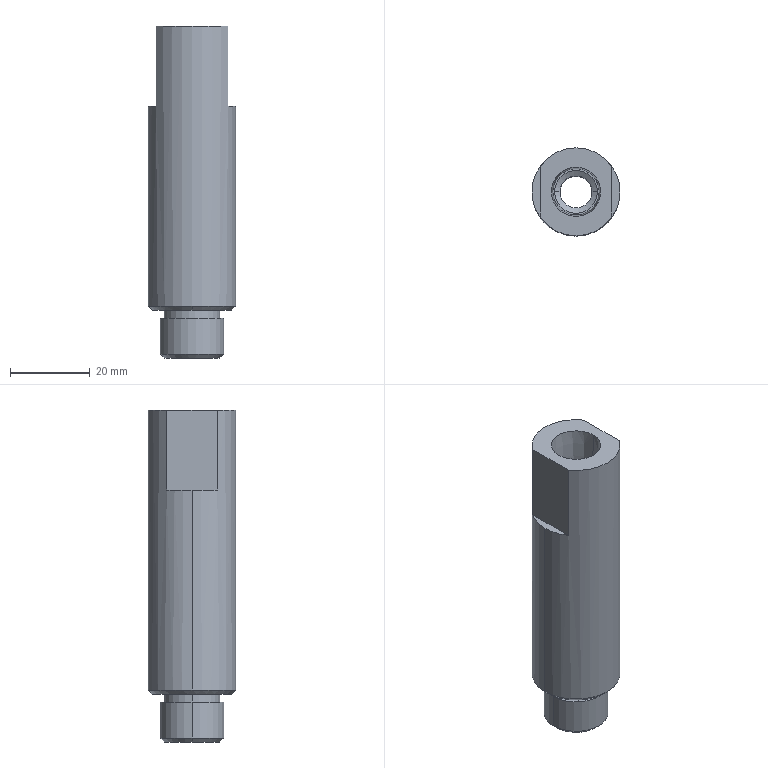Part | SolidWorks | features BaseBody 1 | 1 solid | 27 faces | box 22 x 22 x 83 mm | volume 23413 mm3 | cylinder 10 | plane 9 | cone 8 | commonest cylinder face diameters 8 x2 10.7 x2 14 x2 16 x2 22 x2
STEP:
#1=CARTESIAN_POINT('',(9.,6.325,63.));
#2=VERTEX_POINT('',#1);
#3=CARTESIAN_POINT('',(11.,0.,63.));
#4=VERTEX_POINT('',#3);
#5=CARTESIAN_POINT('',(0.,0.,63.));
#6=DIRECTION('',(0.,0.,-1.));
#7=DIRECTION('',(-1.,0.,0.));
#8=AXIS2_PLACEMENT_3D('',#5,#6,#7);
#9=CIRCLE('',#8,11.);
#10=EDGE_CURVE('',#2,#4,#9,.T.);
#11=ORIENTED_EDGE('',*,*,#10,.T.);
#12=CARTESIAN_POINT('',(11.,0.,13.));
#13=VERTEX_POINT('',#12);
#14=CARTESIAN_POINT('',(11.,0.,83.));
#15=DIRECTION('',(0.,0.,-1.));
#16=VECTOR('',#15,1000.);
#17=LINE('',#14,#16);
#18=EDGE_CURVE('',#4,#13,#17,.T.);
#19=ORIENTED_EDGE('',*,*,#18,.T.);
#20=CARTESIAN_POINT('',(0.,11.,13.));
#21=VERTEX_POINT('',#20);
#22=CARTESIAN_POINT('',(0.,0.,13.));
#23=DIRECTION('',(0.,0.,1.));
#24=DIRECTION('',(-1.,0.,0.));
#25=AXIS2_PLACEMENT_3D('',#22,#23,#24);
#26=CIRCLE('',#25,11.);
#27=EDGE_CURVE('',#13,#21,#26,.T.);
#28=ORIENTED_EDGE('',*,*,#27,.T.);
#29=CARTESIAN_POINT('',(-11.,0.,13.));
#30=VERTEX_POINT('',#29);
#31=CARTESIAN_POINT('',(0.,0.,13.));
#32=DIRECTION('',(0.,0.,1.));
#33=DIRECTION('',(-1.,0.,0.));
#34=AXIS2_PLACEMENT_3D('',#31,#32,#33);
#35=CIRCLE('',#34,11.);
#36=EDGE_CURVE('',#21,#30,#35,.T.);
#37=ORIENTED_EDGE('',*,*,#36,.T.);
#38=CARTESIAN_POINT('',(-11.,0.,63.));
#39=VERTEX_POINT('',#38);
#40=CARTESIAN_POINT('',(-11.,0.,83.));
#41=DIRECTION('',(0.,0.,-1.));
#42=VECTOR('',#41,1000.);
#43=LINE('',#40,#42);
#44=EDGE_CURVE('',#39,#30,#43,.T.);
#45=ORIENTED_EDGE('',*,*,#44,.F.);
#46=CARTESIAN_POINT('',(-9.,6.325,63.));
#47=VERTEX_POINT('',#46);
#48=CARTESIAN_POINT('',(0.,0.,63.));
#49=DIRECTION('',(0.,0.,-1.));
#50=DIRECTION('',(-1.,0.,0.));
#51=AXIS2_PLACEMENT_3D('',#48,#49,#50);
#52=CIRCLE('',#51,11.);
#53=EDGE_CURVE('',#39,#47,#52,.T.);
#54=ORIENTED_EDGE('',*,*,#53,.T.);
#55=CARTESIAN_POINT('',(-9.,6.325,83.));
#56=VERTEX_POINT('',#55);
#57=CARTESIAN_POINT('',(-9.,6.325,83.));
#58=DIRECTION('',(0.,0.,1.));
#59=VECTOR('',#58,1000.);
#60=LINE('',#57,#59);
#61=EDGE_CURVE('',#47,#56,#60,.T.);
#62=ORIENTED_EDGE('',*,*,#61,.T.);
#63=CARTESIAN_POINT('',(9.,6.325,83.));
#64=VERTEX_POINT('',#63);
#65=CARTESIAN_POINT('',(0.,0.,83.));
#66=DIRECTION('',(0.,0.,-1.));
#67=DIRECTION('',(-1.,0.,0.));
#68=AXIS2_PLACEMENT_3D('',#65,#66,#67);
#69=CIRCLE('',#68,11.);
#70=EDGE_CURVE('',#56,#64,#69,.T.);
#71=ORIENTED_EDGE('',*,*,#70,.T.);
#72=CARTESIAN_POINT('',(9.,6.325,83.));
#73=DIRECTION('',(0.,0.,-1.));
#74=VECTOR('',#73,1000.);
#75=LINE('',#72,#74);
#76=EDGE_CURVE('',#64,#2,#75,.T.);
#77=ORIENTED_EDGE('',*,*,#76,.T.);
#78=EDGE_LOOP('',(#11,#19,#28,#37,#45,#54,#62,#71,#77));
#79=FACE_OUTER_BOUND('',#78,.T.);
#80=CARTESIAN_POINT('',(0.,0.,83.));
#81=DIRECTION('',(0.,0.,-1.));
#82=DIRECTION('',(-1.,0.,0.));
#83=AXIS2_PLACEMENT_3D('',#80,#81,#82);
#84=CYLINDRICAL_SURFACE('',#83,11.);
#85=ADVANCED_FACE('',(#79),#84,.T.);
#86=CARTESIAN_POINT('',(0.,-10.,12.));
#87=VERTEX_POINT('',#86);
#88=CARTESIAN_POINT('',(0.,10.,12.));
#89=VERTEX_POINT('',#88);
#90=CARTESIAN_POINT('',(0.,0.,12.));
#91=DIRECTION('',(0.,0.,1.));
#92=DIRECTION('',(0.,-1.,0.));
#93=AXIS2_PLACEMENT_3D('',#90,#91,#92);
#94=CIRCLE('',#93,10.);
#95=EDGE_CURVE('',#87,#89,#94,.T.);
#96=ORIENTED_EDGE('',*,*,#95,.T.);
#97=CARTESIAN_POINT('',(0.,11.,13.));
#98=DIRECTION('',(0.,0.7071,0.7071));
#99=VECTOR('',#98,1000.);
#100=LINE('',#97,#99);
#101=EDGE_CURVE('',#89,#21,#100,.T.);
#102=ORIENTED_EDGE('',*,*,#101,.T.);
#103=ORIENTED_EDGE('',*,*,#27,.F.);
#104=CARTESIAN_POINT('',(0.,-11.,13.));
#105=VERTEX_POINT('',#104);
#106=CARTESIAN_POINT('',(0.,0.,13.));
#107=DIRECTION('',(0.,0.,1.));
#108=DIRECTION('',(-1.,0.,0.));
#109=AXIS2_PLACEMENT_3D('',#106,#107,#108);
#110=CIRCLE('',#109,11.);
#111=EDGE_CURVE('',#105,#13,#110,.T.);
#112=ORIENTED_EDGE('',*,*,#111,.F.);
#113=CARTESIAN_POINT('',(0.,-11.,13.));
#114=DIRECTION('',(0.,-0.7071,0.7071));
#115=VECTOR('',#114,1000.);
#116=LINE('',#113,#115);
#117=EDGE_CURVE('',#87,#105,#116,.T.);
#118=ORIENTED_EDGE('',*,*,#117,.F.);
#119=EDGE_LOOP('',(#96,#102,#103,#112,#118));
#120=FACE_OUTER_BOUND('',#119,.T.);
#121=CARTESIAN_POINT('',(0.,0.,13.));
#122=DIRECTION('',(0.,0.,1.));
#123=DIRECTION('',(0.,-1.,0.));
#124=AXIS2_PLACEMENT_3D('',#121,#122,#123);
#125=CONICAL_SURFACE('',#124,11.,0.7854);
#126=ADVANCED_FACE('',(#120),#125,.T.);
#127=CARTESIAN_POINT('',(-5.811,0.,72.));
#128=VERTEX_POINT('',#127);
#129=CARTESIAN_POINT('',(5.811,0.,72.));
#130=VERTEX_POINT('',#129);
#131=CARTESIAN_POINT('',(0.,0.,72.));
#132=DIRECTION('',(0.,0.,1.));
#133=DIRECTION('',(1.,0.,0.));
#134=AXIS2_PLACEMENT_3D('',#131,#132,#133);
#135=CIRCLE('',#134,5.811);
#136=EDGE_CURVE('',#128,#130,#135,.T.);
#137=ORIENTED_EDGE('',*,*,#136,.F.);
#138=CARTESIAN_POINT('',(-6.154,0.,83.));
#139=VERTEX_POINT('',#138);
#140=CARTESIAN_POINT('',(-6.154,0.,83.));
#141=DIRECTION('',(-0.0312,0.,0.9995));
#142=VECTOR('',#141,1000.);
#143=LINE('',#140,#142);
#144=EDGE_CURVE('',#128,#139,#143,.T.);
#145=ORIENTED_EDGE('',*,*,#144,.T.);
#146=CARTESIAN_POINT('',(6.154,0.,83.));
#147=VERTEX_POINT('',#146);
#148=CARTESIAN_POINT('',(0.,0.,83.));
#149=DIRECTION('',(0.,0.,-1.));
#150=DIRECTION('',(1.,0.,0.));
#151=AXIS2_PLACEMENT_3D('',#148,#149,#150);
#152=CIRCLE('',#151,6.154);
#153=EDGE_CURVE('',#147,#139,#152,.T.);
#154=ORIENTED_EDGE('',*,*,#153,.F.);
#155=CARTESIAN_POINT('',(6.154,0.,83.));
#156=DIRECTION('',(0.0312,0.,0.9995));
#157=VECTOR('',#156,1000.);
#158=LINE('',#155,#157);
#159=EDGE_CURVE('',#130,#147,#158,.T.);
#160=ORIENTED_EDGE('',*,*,#159,.F.);
#161=EDGE_LOOP('',(#137,#145,#154,#160));
#162=FACE_OUTER_BOUND('',#161,.T.);
#163=CARTESIAN_POINT('',(0.,0.,83.));
#164=DIRECTION('',(0.,0.,1.));
#165=DIRECTION('',(1.,0.,0.));
#166=AXIS2_PLACEMENT_3D('',#163,#164,#165);
#167=CONICAL_SURFACE('',#166,6.154,0.03121);
#168=ADVANCED_FACE('',(#162),#167,.F.);
#169=CARTESIAN_POINT('',(-7.,0.,12.));
#170=VERTEX_POINT('',#169);
#171=CARTESIAN_POINT('',(7.,0.,12.));
#172=VERTEX_POINT('',#171);
#173=CARTESIAN_POINT('',(0.,0.,12.));
#174=DIRECTION('',(0.,0.,-1.));
#175=DIRECTION('',(-1.,0.,0.));
#176=AXIS2_PLACEMENT_3D('',#173,#174,#175);
#177=CIRCLE('',#176,7.);
#178=EDGE_CURVE('',#170,#172,#177,.T.);
#179=ORIENTED_EDGE('',*,*,#178,.T.);
#180=CARTESIAN_POINT('',(7.,0.,10.));
#181=VERTEX_POINT('',#180);
#182=CARTESIAN_POINT('',(7.,0.,0.));
#183=DIRECTION('',(0.,0.,-1.));
#184=VECTOR('',#183,1000.);
#185=LINE('',#182,#184);
#186=EDGE_CURVE('',#172,#181,#185,.T.);
#187=ORIENTED_EDGE('',*,*,#186,.T.);
#188=CARTESIAN_POINT('',(-7.,0.,10.));
#189=VERTEX_POINT('',#188);
#190=CARTESIAN_POINT('',(0.,0.,10.));
#191=DIRECTION('',(0.,0.,1.));
#192=DIRECTION('',(-1.,0.,0.));
#193=AXIS2_PLACEMENT_3D('',#190,#191,#192);
#194=CIRCLE('',#193,7.);
#195=EDGE_CURVE('',#181,#189,#194,.T.);
#196=ORIENTED_EDGE('',*,*,#195,.T.);
#197=CARTESIAN_POINT('',(-7.,0.,0.));
#198=DIRECTION('',(0.,0.,-1.));
#199=VECTOR('',#198,1000.);
#200=LINE('',#197,#199);
#201=EDGE_CURVE('',#170,#189,#200,.T.);
#202=ORIENTED_EDGE('',*,*,#201,.F.);
#203=EDGE_LOOP('',(#179,#187,#196,#202));
#204=FACE_OUTER_BOUND('',#203,.T.);
#205=CARTESIAN_POINT('',(0.,0.,0.));
#206=DIRECTION('',(0.,0.,-1.));
#207=DIRECTION('',(-1.,0.,0.));
#208=AXIS2_PLACEMENT_3D('',#205,#206,#207);
#209=CYLINDRICAL_SURFACE('',#208,7.);
#210=ADVANCED_FACE('',(#204),#209,.T.);
#211=CARTESIAN_POINT('',(-5.35,0.,65.));
#212=VERTEX_POINT('',#211);
#213=CARTESIAN_POINT('',(5.35,0.,65.));
#214=VERTEX_POINT('',#213);
#215=CARTESIAN_POINT('',(0.,0.,65.));
#216=DIRECTION('',(0.,0.,1.));
#217=DIRECTION('',(1.,0.,0.));
#218=AXIS2_PLACEMENT_3D('',#215,#216,#217);
#219=CIRCLE('',#218,5.35);
#220=EDGE_CURVE('',#212,#214,#219,.T.);
#221=ORIENTED_EDGE('',*,*,#220,.F.);
#222=CARTESIAN_POINT('',(-5.35,0.,72.));
#223=VERTEX_POINT('',#222);
#224=CARTESIAN_POINT('',(-5.35,0.,83.));
#225=DIRECTION('',(0.,0.,1.));
#226=VECTOR('',#225,1000.);
#227=LINE('',#224,#226);
#228=EDGE_CURVE('',#212,#223,#227,.T.);
#229=ORIENTED_EDGE('',*,*,#228,.T.);
#230=CARTESIAN_POINT('',(5.35,0.,72.));
#231=VERTEX_POINT('',#230);
#232=CARTESIAN_POINT('',(0.,0.,72.));
#233=DIRECTION('',(0.,0.,1.));
#234=DIRECTION('',(1.,0.,0.));
#235=AXIS2_PLACEMENT_3D('',#232,#233,#234);
#236=CIRCLE('',#235,5.35);
#237=EDGE_CURVE('',#223,#231,#236,.T.);
#238=ORIENTED_EDGE('',*,*,#237,.T.);
#239=CARTESIAN_POINT('',(5.35,0.,83.));
#240=DIRECTION('',(0.,0.,1.));
#241=VECTOR('',#240,1000.);
#242=LINE('',#239,#241);
#243=EDGE_CURVE('',#214,#231,#242,.T.);
#244=ORIENTED_EDGE('',*,*,#243,.F.);
#245=EDGE_LOOP('',(#221,#229,#238,#244));
#246=FACE_OUTER_BOUND('',#245,.T.);
#247=CARTESIAN_POINT('',(0.,0.,83.));
#248=DIRECTION('',(0.,0.,1.));
#249=DIRECTION('',(1.,0.,0.));
#250=AXIS2_PLACEMENT_3D('',#247,#248,#249);
#251=CYLINDRICAL_SURFACE('',#250,5.35);
#252=ADVANCED_FACE('',(#246),#251,.F.);
#253=CARTESIAN_POINT('',(-4.,0.,64.189));
#254=VERTEX_POINT('',#253);
#255=CARTESIAN_POINT('',(4.,0.,64.189));
#256=VERTEX_POINT('',#255);
#257=CARTESIAN_POINT('',(0.,0.,64.189));
#258=DIRECTION('',(0.,0.,1.));
#259=DIRECTION('',(1.,0.,0.));
#260=AXIS2_PLACEMENT_3D('',#257,#258,#259);
#261=CIRCLE('',#260,4.);
#262=EDGE_CURVE('',#254,#256,#261,.T.);
#263=ORIENTED_EDGE('',*,*,#262,.F.);
#264=CARTESIAN_POINT('',(-5.35,0.,65.));
#265=DIRECTION('',(-0.8572,0.,0.515));
#266=VECTOR('',#265,1000.);
#267=LINE('',#264,#266);
#268=EDGE_CURVE('',#254,#212,#267,.T.);
#269=ORIENTED_EDGE('',*,*,#268,.T.);
#270=ORIENTED_EDGE('',*,*,#220,.T.);
#271=CARTESIAN_POINT('',(5.35,0.,65.));
#272=DIRECTION('',(0.8572,0.,0.515));
#273=VECTOR('',#272,1000.);
#274=LINE('',#271,#273);
#275=EDGE_CURVE('',#256,#214,#274,.T.);
#276=ORIENTED_EDGE('',*,*,#275,.F.);
#277=EDGE_LOOP('',(#263,#269,#270,#276));
#278=FACE_OUTER_BOUND('',#277,.T.);
#279=CARTESIAN_POINT('',(0.,0.,65.));
#280=DIRECTION('',(0.,0.,1.));
#281=DIRECTION('',(1.,0.,0.));
#282=AXIS2_PLACEMENT_3D('',#279,#280,#281);
#283=CONICAL_SURFACE('',#282,5.35,1.03);
#284=ADVANCED_FACE('',(#278),#283,.F.);
#285=CARTESIAN_POINT('',(8.,0.,10.));
#286=VERTEX_POINT('',#285);
#287=CARTESIAN_POINT('',(-8.,0.,10.));
#288=VERTEX_POINT('',#287);
#289=CARTESIAN_POINT('',(0.,0.,10.));
#290=DIRECTION('',(0.,0.,1.));
#291=DIRECTION('',(-1.,0.,0.));
#292=AXIS2_PLACEMENT_3D('',#289,#290,#291);
#293=CIRCLE('',#292,8.);
#294=EDGE_CURVE('',#286,#288,#293,.T.);
#295=ORIENTED_EDGE('',*,*,#294,.F.);
#296=CARTESIAN_POINT('',(8.,0.,1.));
#297=VERTEX_POINT('',#296);
#298=CARTESIAN_POINT('',(8.,0.,12.));
#299=DIRECTION('',(0.,0.,-1.));
#300=VECTOR('',#299,1000.);
#301=LINE('',#298,#300);
#302=EDGE_CURVE('',#286,#297,#301,.T.);
#303=ORIENTED_EDGE('',*,*,#302,.T.);
#304=CARTESIAN_POINT('',(-8.,0.,1.));
#305=VERTEX_POINT('',#304);
#306=CARTESIAN_POINT('',(0.,0.,1.));
#307=DIRECTION('',(0.,0.,1.));
#308=DIRECTION('',(-1.,0.,0.));
#309=AXIS2_PLACEMENT_3D('',#306,#307,#308);
#310=CIRCLE('',#309,8.);
#311=EDGE_CURVE('',#297,#305,#310,.T.);
#312=ORIENTED_EDGE('',*,*,#311,.T.);
#313=CARTESIAN_POINT('',(-8.,0.,12.));
#314=DIRECTION('',(0.,0.,-1.));
#315=VECTOR('',#314,1000.);
#316=LINE('',#313,#315);
#317=EDGE_CURVE('',#288,#305,#316,.T.);
#318=ORIENTED_EDGE('',*,*,#317,.F.);
#319=EDGE_LOOP('',(#295,#303,#312,#318));
#320=FACE_OUTER_BOUND('',#319,.T.);
#321=CARTESIAN_POINT('',(0.,0.,12.));
#322=DIRECTION('',(0.,0.,-1.));
#323=DIRECTION('',(-1.,0.,0.));
#324=AXIS2_PLACEMENT_3D('',#321,#322,#323);
#325=CYLINDRICAL_SURFACE('',#324,8.);
#326=ADVANCED_FACE('',(#320),#325,.T.);
#327=ORIENTED_EDGE('',*,*,#262,.T.);
#328=CARTESIAN_POINT('',(4.,0.,0.));
#329=VERTEX_POINT('',#328);
#330=CARTESIAN_POINT('',(4.,0.,0.));
#331=DIRECTION('',(0.,0.,-1.));
#332=VECTOR('',#331,1000.);
#333=LINE('',#330,#332);
#334=EDGE_CURVE('',#256,#329,#333,.T.);
#335=ORIENTED_EDGE('',*,*,#334,.T.);
#336=CARTESIAN_POINT('',(-4.,0.,0.));
#337=VERTEX_POINT('',#336);
#338=CARTESIAN_POINT('',(0.,0.,0.));
#339=DIRECTION('',(0.,0.,1.));
#340=DIRECTION('',(-1.,0.,0.));
#341=AXIS2_PLACEMENT_3D('',#338,#339,#340);
#342=CIRCLE('',#341,4.);
#343=EDGE_CURVE('',#337,#329,#342,.T.);
#344=ORIENTED_EDGE('',*,*,#343,.F.);
#345=CARTESIAN_POINT('',(-4.,0.,0.));
#346=DIRECTION('',(0.,0.,-1.));
#347=VECTOR('',#346,1000.);
#348=LINE('',#345,#347);
#349=EDGE_CURVE('',#254,#337,#348,.T.);
#350=ORIENTED_EDGE('',*,*,#349,.F.);
#351=EDGE_LOOP('',(#327,#335,#344,#350));
#352=FACE_OUTER_BOUND('',#351,.T.);
#353=CARTESIAN_POINT('',(0.,0.,0.));
#354=DIRECTION('',(0.,0.,-1.));
#355=DIRECTION('',(-1.,0.,0.));
#356=AXIS2_PLACEMENT_3D('',#353,#354,#355);
#357=CYLINDRICAL_SURFACE('',#356,4.);
#358=ADVANCED_FACE('',(#352),#357,.F.);
#359=CARTESIAN_POINT('',(7.,0.,0.));
#360=VERTEX_POINT('',#359);
#361=CARTESIAN_POINT('',(-7.,0.,0.));
#362=VERTEX_POINT('',#361);
#363=CARTESIAN_POINT('',(0.,0.,0.));
#364=DIRECTION('',(0.,0.,1.));
#365=DIRECTION('',(1.,0.,0.));
#366=AXIS2_PLACEMENT_3D('',#363,#364,#365);
#367=CIRCLE('',#366,7.);
#368=EDGE_CURVE('',#360,#362,#367,.T.);
#369=ORIENTED_EDGE('',*,*,#368,.T.);
#370=CARTESIAN_POINT('',(-8.,0.,1.));
#371=DIRECTION('',(-0.7071,0.,0.7071));
#372=VECTOR('',#371,1000.);
#373=LINE('',#370,#372);
#374=EDGE_CURVE('',#362,#305,#373,.T.);
#375=ORIENTED_EDGE('',*,*,#374,.T.);
#376=ORIENTED_EDGE('',*,*,#311,.F.);
#377=CARTESIAN_POINT('',(8.,0.,1.));
#378=DIRECTION('',(0.7071,0.,0.7071));
#379=VECTOR('',#378,1000.);
#380=LINE('',#377,#379);
#381=EDGE_CURVE('',#360,#297,#380,.T.);
#382=ORIENTED_EDGE('',*,*,#381,.F.);
#383=EDGE_LOOP('',(#369,#375,#376,#382));
#384=FACE_OUTER_BOUND('',#383,.T.);
#385=CARTESIAN_POINT('',(0.,0.,1.));
#386=DIRECTION('',(0.,0.,1.));
#387=DIRECTION('',(1.,0.,0.));
#388=AXIS2_PLACEMENT_3D('',#385,#386,#387);
#389=CONICAL_SURFACE('',#388,8.,0.7854);
#390=ADVANCED_FACE('',(#384),#389,.T.);
#391=ORIENTED_EDGE('',*,*,#18,.F.);
#392=CARTESIAN_POINT('',(9.,-6.325,63.));
#393=VERTEX_POINT('',#392);
#394=CARTESIAN_POINT('',(0.,0.,63.));
#395=DIRECTION('',(0.,0.,-1.));
#396=DIRECTION('',(-1.,0.,0.));
#397=AXIS2_PLACEMENT_3D('',#394,#395,#396);
#398=CIRCLE('',#397,11.);
#399=EDGE_CURVE('',#4,#393,#398,.T.);
#400=ORIENTED_EDGE('',*,*,#399,.T.);
#401=CARTESIAN_POINT('',(9.,-6.325,83.));
#402=VERTEX_POINT('',#401);
#403=CARTESIAN_POINT('',(9.,-6.325,63.));
#404=DIRECTION('',(0.,0.,-1.));
#405=VECTOR('',#404,1000.);
#406=LINE('',#403,#405);
#407=EDGE_CURVE('',#402,#393,#406,.T.);
#408=ORIENTED_EDGE('',*,*,#407,.F.);
#409=CARTESIAN_POINT('',(-9.,-6.325,83.));
#410=VERTEX_POINT('',#409);
#411=CARTESIAN_POINT('',(0.,0.,83.));
#412=DIRECTION('',(0.,0.,1.));
#413=DIRECTION('',(-1.,0.,0.));
#414=AXIS2_PLACEMENT_3D('',#411,#412,#413);
#415=CIRCLE('',#414,11.);
#416=EDGE_CURVE('',#410,#402,#415,.T.);
#417=ORIENTED_EDGE('',*,*,#416,.F.);
#418=CARTESIAN_POINT('',(-9.,-6.325,63.));
#419=VERTEX_POINT('',#418);
#420=CARTESIAN_POINT('',(-9.,-6.325,63.));
#421=DIRECTION('',(0.,0.,1.));
#422=VECTOR('',#421,1000.);
#423=LINE('',#420,#422);
#424=EDGE_CURVE('',#419,#410,#423,.T.);
#425=ORIENTED_EDGE('',*,*,#424,.F.);
#426=CARTESIAN_POINT('',(0.,0.,63.));
#427=DIRECTION('',(0.,0.,-1.));
#428=DIRECTION('',(-1.,0.,0.));
#429=AXIS2_PLACEMENT_3D('',#426,#427,#428);
#430=CIRCLE('',#429,11.);
#431=EDGE_CURVE('',#419,#39,#430,.T.);
#432=ORIENTED_EDGE('',*,*,#431,.T.);
#433=ORIENTED_EDGE('',*,*,#44,.T.);
#434=CARTESIAN_POINT('',(0.,0.,13.));
#435=DIRECTION('',(0.,0.,1.));
#436=DIRECTION('',(-1.,0.,0.));
#437=AXIS2_PLACEMENT_3D('',#434,#435,#436);
#438=CIRCLE('',#437,11.);
#439=EDGE_CURVE('',#30,#105,#438,.T.);
#440=ORIENTED_EDGE('',*,*,#439,.T.);
#441=ORIENTED_EDGE('',*,*,#111,.T.);
#442=EDGE_LOOP('',(#391,#400,#408,#417,#425,#432,#433,#440,#441));
#443=FACE_OUTER_BOUND('',#442,.T.);
#444=CARTESIAN_POINT('',(0.,0.,83.));
#445=DIRECTION('',(0.,0.,-1.));
#446=DIRECTION('',(-1.,0.,0.));
#447=AXIS2_PLACEMENT_3D('',#444,#445,#446);
#448=CYLINDRICAL_SURFACE('',#447,11.);
#449=ADVANCED_FACE('',(#443),#448,.T.);
#450=ORIENTED_EDGE('',*,*,#76,.F.);
#451=CARTESIAN_POINT('',(9.,12.5,83.));
#452=DIRECTION('',(0.,-1.,0.));
#453=VECTOR('',#452,1000.);
#454=LINE('',#451,#453);
#455=EDGE_CURVE('',#64,#402,#454,.T.);
#456=ORIENTED_EDGE('',*,*,#455,.T.);
#457=ORIENTED_EDGE('',*,*,#407,.T.);
#458=CARTESIAN_POINT('',(9.,12.5,63.));
#459=DIRECTION('',(0.,1.,0.));
#460=VECTOR('',#459,1000.);
#461=LINE('',#458,#460);
#462=EDGE_CURVE('',#393,#2,#461,.T.);
#463=ORIENTED_EDGE('',*,*,#462,.T.);
#464=EDGE_LOOP('',(#450,#456,#457,#463));
#465=FACE_OUTER_BOUND('',#464,.T.);
#466=CARTESIAN_POINT('',(9.,12.5,63.));
#467=DIRECTION('',(1.,0.,0.));
#468=DIRECTION('',(0.,1.,0.));
#469=AXIS2_PLACEMENT_3D('',#466,#467,#468);
#470=PLANE('',#469);
#471=ADVANCED_FACE('',(#465),#470,.T.);
#472=ORIENTED_EDGE('',*,*,#70,.F.);
#473=CARTESIAN_POINT('',(-9.,0.,83.));
#474=DIRECTION('',(0.,-1.,0.));
#475=VECTOR('',#474,1000.);
#476=LINE('',#473,#475);
#477=EDGE_CURVE('',#56,#410,#476,.T.);
#478=ORIENTED_EDGE('',*,*,#477,.T.);
#479=ORIENTED_EDGE('',*,*,#416,.T.);
#480=ORIENTED_EDGE('',*,*,#455,.F.);
#481=EDGE_LOOP('',(#472,#478,#479,#480));
#482=FACE_OUTER_BOUND('',#481,.T.);
#483=ORIENTED_EDGE('',*,*,#153,.T.);
#484=CARTESIAN_POINT('',(0.,0.,83.));
#485=DIRECTION('',(0.,0.,-1.));
#486=DIRECTION('',(1.,0.,0.));
#487=AXIS2_PLACEMENT_3D('',#484,#485,#486);
#488=CIRCLE('',#487,6.154);
#489=EDGE_CURVE('',#139,#147,#488,.T.);
#490=ORIENTED_EDGE('',*,*,#489,.T.);
#491=EDGE_LOOP('',(#483,#490));
#492=FACE_BOUND('',#491,.T.);
#493=CARTESIAN_POINT('',(0.,0.,83.));
#494=DIRECTION('',(0.,0.,1.));
#495=DIRECTION('',(1.,0.,0.));
#496=AXIS2_PLACEMENT_3D('',#493,#494,#495);
#497=PLANE('',#496);
#498=ADVANCED_FACE('',(#482,#492),#497,.T.);
#499=ORIENTED_EDGE('',*,*,#424,.T.);
#500=ORIENTED_EDGE('',*,*,#477,.F.);
#501=ORIENTED_EDGE('',*,*,#61,.F.);
#502=CARTESIAN_POINT('',(-9.,12.5,63.));
#503=DIRECTION('',(0.,-1.,0.));
#504=VECTOR('',#503,1000.);
#505=LINE('',#502,#504);
#506=EDGE_CURVE('',#47,#419,#505,.T.);
#507=ORIENTED_EDGE('',*,*,#506,.T.);
#508=EDGE_LOOP('',(#499,#500,#501,#507));
#509=FACE_OUTER_BOUND('',#508,.T.);
#510=CARTESIAN_POINT('',(-9.,12.5,63.));
#511=DIRECTION('',(-1.,0.,0.));
#512=DIRECTION('',(0.,-1.,0.));
#513=AXIS2_PLACEMENT_3D('',#510,#511,#512);
#514=PLANE('',#513);
#515=ADVANCED_FACE('',(#509),#514,.T.);
#516=ORIENTED_EDGE('',*,*,#431,.F.);
#517=ORIENTED_EDGE('',*,*,#506,.F.);
#518=ORIENTED_EDGE('',*,*,#53,.F.);
#519=EDGE_LOOP('',(#516,#517,#518));
#520=FACE_OUTER_BOUND('',#519,.T.);
#521=CARTESIAN_POINT('',(0.,0.,63.));
#522=DIRECTION('',(0.,0.,1.));
#523=DIRECTION('',(1.,0.,0.));
#524=AXIS2_PLACEMENT_3D('',#521,#522,#523);
#525=PLANE('',#524);
#526=ADVANCED_FACE('',(#520),#525,.T.);
#527=ORIENTED_EDGE('',*,*,#101,.F.);
#528=CARTESIAN_POINT('',(0.,0.,12.));
#529=DIRECTION('',(0.,0.,1.));
#530=DIRECTION('',(0.,-1.,0.));
#531=AXIS2_PLACEMENT_3D('',#528,#529,#530);
#532=CIRCLE('',#531,10.);
#533=EDGE_CURVE('',#89,#87,#532,.T.);
#534=ORIENTED_EDGE('',*,*,#533,.T.);
#535=ORIENTED_EDGE('',*,*,#117,.T.);
#536=ORIENTED_EDGE('',*,*,#439,.F.);
#537=ORIENTED_EDGE('',*,*,#36,.F.);
#538=EDGE_LOOP('',(#527,#534,#535,#536,#537));
#539=FACE_OUTER_BOUND('',#538,.T.);
#540=CARTESIAN_POINT('',(0.,0.,13.));
#541=DIRECTION('',(0.,0.,1.));
#542=DIRECTION('',(0.,-1.,0.));
#543=AXIS2_PLACEMENT_3D('',#540,#541,#542);
#544=CONICAL_SURFACE('',#543,11.,0.7854);
#545=ADVANCED_FACE('',(#539),#544,.T.);
#546=ORIENTED_EDGE('',*,*,#10,.F.);
#547=ORIENTED_EDGE('',*,*,#462,.F.);
#548=ORIENTED_EDGE('',*,*,#399,.F.);
#549=EDGE_LOOP('',(#546,#547,#548));
#550=FACE_OUTER_BOUND('',#549,.T.);
#551=CARTESIAN_POINT('',(0.,0.,63.));
#552=DIRECTION('',(0.,0.,1.));
#553=DIRECTION('',(1.,0.,0.));
#554=AXIS2_PLACEMENT_3D('',#551,#552,#553);
#555=PLANE('',#554);
#556=ADVANCED_FACE('',(#550),#555,.T.);
#557=ORIENTED_EDGE('',*,*,#144,.F.);
#558=CARTESIAN_POINT('',(0.,0.,72.));
#559=DIRECTION('',(0.,0.,1.));
#560=DIRECTION('',(1.,0.,0.));
#561=AXIS2_PLACEMENT_3D('',#558,#559,#560);
#562=CIRCLE('',#561,5.811);
#563=EDGE_CURVE('',#130,#128,#562,.T.);
#564=ORIENTED_EDGE('',*,*,#563,.F.);
#565=ORIENTED_EDGE('',*,*,#159,.T.);
#566=ORIENTED_EDGE('',*,*,#489,.F.);
#567=EDGE_LOOP('',(#557,#564,#565,#566));
#568=FACE_OUTER_BOUND('',#567,.T.);
#569=CARTESIAN_POINT('',(0.,0.,83.));
#570=DIRECTION('',(0.,0.,1.));
#571=DIRECTION('',(1.,0.,0.));
#572=AXIS2_PLACEMENT_3D('',#569,#570,#571);
#573=CONICAL_SURFACE('',#572,6.154,0.03121);
#574=ADVANCED_FACE('',(#568),#573,.F.);
#575=ORIENTED_EDGE('',*,*,#178,.F.);
#576=CARTESIAN_POINT('',(0.,0.,12.));
#577=DIRECTION('',(0.,0.,-1.));
#578=DIRECTION('',(-1.,0.,0.));
#579=AXIS2_PLACEMENT_3D('',#576,#577,#578);
#580=CIRCLE('',#579,7.);
#581=EDGE_CURVE('',#172,#170,#580,.T.);
#582=ORIENTED_EDGE('',*,*,#581,.F.);
#583=EDGE_LOOP('',(#575,#582));
#584=FACE_BOUND('',#583,.T.);
#585=ORIENTED_EDGE('',*,*,#95,.F.);
#586=ORIENTED_EDGE('',*,*,#533,.F.);
#587=EDGE_LOOP('',(#585,#586));
#588=FACE_OUTER_BOUND('',#587,.T.);
#589=CARTESIAN_POINT('',(0.,0.,12.));
#590=DIRECTION('',(0.,0.,1.));
#591=DIRECTION('',(1.,0.,0.));
#592=AXIS2_PLACEMENT_3D('',#589,#590,#591);
#593=PLANE('',#592);
#594=ADVANCED_FACE('',(#584,#588),#593,.F.);
#595=ORIENTED_EDGE('',*,*,#563,.T.);
#596=ORIENTED_EDGE('',*,*,#136,.T.);
#597=EDGE_LOOP('',(#595,#596));
#598=FACE_OUTER_BOUND('',#597,.T.);
#599=CARTESIAN_POINT('',(0.,0.,72.));
#600=DIRECTION('',(0.,0.,1.));
#601=DIRECTION('',(1.,0.,0.));
#602=AXIS2_PLACEMENT_3D('',#599,#600,#601);
#603=CIRCLE('',#602,5.35);
#604=EDGE_CURVE('',#231,#223,#603,.T.);
#605=ORIENTED_EDGE('',*,*,#604,.F.);
#606=ORIENTED_EDGE('',*,*,#237,.F.);
#607=EDGE_LOOP('',(#605,#606));
#608=FACE_BOUND('',#607,.T.);
#609=CARTESIAN_POINT('',(5.35,0.,72.));
#610=DIRECTION('',(0.,0.,-1.));
#611=DIRECTION('',(-1.,0.,0.));
#612=AXIS2_PLACEMENT_3D('',#609,#610,#611);
#613=PLANE('',#612);
#614=ADVANCED_FACE('',(#598,#608),#613,.F.);
#615=ORIENTED_EDGE('',*,*,#186,.F.);
#616=ORIENTED_EDGE('',*,*,#581,.T.);
#617=ORIENTED_EDGE('',*,*,#201,.T.);
#618=CARTESIAN_POINT('',(0.,0.,10.));
#619=DIRECTION('',(0.,0.,1.));
#620=DIRECTION('',(-1.,0.,0.));
#621=AXIS2_PLACEMENT_3D('',#618,#619,#620);
#622=CIRCLE('',#621,7.);
#623=EDGE_CURVE('',#189,#181,#622,.T.);
#624=ORIENTED_EDGE('',*,*,#623,.T.);
#625=EDGE_LOOP('',(#615,#616,#617,#624));
#626=FACE_OUTER_BOUND('',#625,.T.);
#627=CARTESIAN_POINT('',(0.,0.,0.));
#628=DIRECTION('',(0.,0.,-1.));
#629=DIRECTION('',(-1.,0.,0.));
#630=AXIS2_PLACEMENT_3D('',#627,#628,#629);
#631=CYLINDRICAL_SURFACE('',#630,7.);
#632=ADVANCED_FACE('',(#626),#631,.T.);
#633=ORIENTED_EDGE('',*,*,#228,.F.);
#634=CARTESIAN_POINT('',(0.,0.,65.));
#635=DIRECTION('',(0.,0.,1.));
#636=DIRECTION('',(1.,0.,0.));
#637=AXIS2_PLACEMENT_3D('',#634,#635,#636);
#638=CIRCLE('',#637,5.35);
#639=EDGE_CURVE('',#214,#212,#638,.T.);
#640=ORIENTED_EDGE('',*,*,#639,.F.);
#641=ORIENTED_EDGE('',*,*,#243,.T.);
#642=ORIENTED_EDGE('',*,*,#604,.T.);
#643=EDGE_LOOP('',(#633,#640,#641,#642));
#644=FACE_OUTER_BOUND('',#643,.T.);
#645=CARTESIAN_POINT('',(0.,0.,83.));
#646=DIRECTION('',(0.,0.,1.));
#647=DIRECTION('',(1.,0.,0.));
#648=AXIS2_PLACEMENT_3D('',#645,#646,#647);
#649=CYLINDRICAL_SURFACE('',#648,5.35);
#650=ADVANCED_FACE('',(#644),#649,.F.);
#651=CARTESIAN_POINT('',(0.,0.,10.));
#652=DIRECTION('',(0.,0.,1.));
#653=DIRECTION('',(-1.,0.,0.));
#654=AXIS2_PLACEMENT_3D('',#651,#652,#653);
#655=CIRCLE('',#654,8.);
#656=EDGE_CURVE('',#288,#286,#655,.T.);
#657=ORIENTED_EDGE('',*,*,#656,.T.);
#658=ORIENTED_EDGE('',*,*,#294,.T.);
#659=EDGE_LOOP('',(#657,#658));
#660=FACE_OUTER_BOUND('',#659,.T.);
#661=ORIENTED_EDGE('',*,*,#623,.F.);
#662=ORIENTED_EDGE('',*,*,#195,.F.);
#663=EDGE_LOOP('',(#661,#662));
#664=FACE_BOUND('',#663,.T.);
#665=CARTESIAN_POINT('',(8.,0.,10.));
#666=DIRECTION('',(0.,0.,1.));
#667=DIRECTION('',(1.,0.,0.));
#668=AXIS2_PLACEMENT_3D('',#665,#666,#667);
#669=PLANE('',#668);
#670=ADVANCED_FACE('',(#660,#664),#669,.T.);
#671=ORIENTED_EDGE('',*,*,#268,.F.);
#672=CARTESIAN_POINT('',(0.,0.,64.189));
#673=DIRECTION('',(0.,0.,1.));
#674=DIRECTION('',(1.,0.,0.));
#675=AXIS2_PLACEMENT_3D('',#672,#673,#674);
#676=CIRCLE('',#675,4.);
#677=EDGE_CURVE('',#256,#254,#676,.T.);
#678=ORIENTED_EDGE('',*,*,#677,.F.);
#679=ORIENTED_EDGE('',*,*,#275,.T.);
#680=ORIENTED_EDGE('',*,*,#639,.T.);
#681=EDGE_LOOP('',(#671,#678,#679,#680));
#682=FACE_OUTER_BOUND('',#681,.T.);
#683=CARTESIAN_POINT('',(0.,0.,65.));
#684=DIRECTION('',(0.,0.,1.));
#685=DIRECTION('',(1.,0.,0.));
#686=AXIS2_PLACEMENT_3D('',#683,#684,#685);
#687=CONICAL_SURFACE('',#686,5.35,1.03);
#688=ADVANCED_FACE('',(#682),#687,.F.);
#689=ORIENTED_EDGE('',*,*,#302,.F.);
#690=ORIENTED_EDGE('',*,*,#656,.F.);
#691=ORIENTED_EDGE('',*,*,#317,.T.);
#692=CARTESIAN_POINT('',(0.,0.,1.));
#693=DIRECTION('',(0.,0.,1.));
#694=DIRECTION('',(-1.,0.,0.));
#695=AXIS2_PLACEMENT_3D('',#692,#693,#694);
#696=CIRCLE('',#695,8.);
#697=EDGE_CURVE('',#305,#297,#696,.T.);
#698=ORIENTED_EDGE('',*,*,#697,.T.);
#699=EDGE_LOOP('',(#689,#690,#691,#698));
#700=FACE_OUTER_BOUND('',#699,.T.);
#701=CARTESIAN_POINT('',(0.,0.,12.));
#702=DIRECTION('',(0.,0.,-1.));
#703=DIRECTION('',(-1.,0.,0.));
#704=AXIS2_PLACEMENT_3D('',#701,#702,#703);
#705=CYLINDRICAL_SURFACE('',#704,8.);
#706=ADVANCED_FACE('',(#700),#705,.T.);
#707=ORIENTED_EDGE('',*,*,#334,.F.);
#708=ORIENTED_EDGE('',*,*,#677,.T.);
#709=ORIENTED_EDGE('',*,*,#349,.T.);
#710=CARTESIAN_POINT('',(0.,0.,0.));
#711=DIRECTION('',(0.,0.,1.));
#712=DIRECTION('',(-1.,0.,0.));
#713=AXIS2_PLACEMENT_3D('',#710,#711,#712);
#714=CIRCLE('',#713,4.);
#715=EDGE_CURVE('',#329,#337,#714,.T.);
#716=ORIENTED_EDGE('',*,*,#715,.F.);
#717=EDGE_LOOP('',(#707,#708,#709,#716));
#718=FACE_OUTER_BOUND('',#717,.T.);
#719=CARTESIAN_POINT('',(0.,0.,0.));
#720=DIRECTION('',(0.,0.,-1.));
#721=DIRECTION('',(-1.,0.,0.));
#722=AXIS2_PLACEMENT_3D('',#719,#720,#721);
#723=CYLINDRICAL_SURFACE('',#722,4.);
#724=ADVANCED_FACE('',(#718),#723,.F.);
#725=ORIENTED_EDGE('',*,*,#374,.F.);
#726=CARTESIAN_POINT('',(0.,0.,0.));
#727=DIRECTION('',(0.,0.,1.));
#728=DIRECTION('',(1.,0.,0.));
#729=AXIS2_PLACEMENT_3D('',#726,#727,#728);
#730=CIRCLE('',#729,7.);
#731=EDGE_CURVE('',#362,#360,#730,.T.);
#732=ORIENTED_EDGE('',*,*,#731,.T.);
#733=ORIENTED_EDGE('',*,*,#381,.T.);
#734=ORIENTED_EDGE('',*,*,#697,.F.);
#735=EDGE_LOOP('',(#725,#732,#733,#734));
#736=FACE_OUTER_BOUND('',#735,.T.);
#737=CARTESIAN_POINT('',(0.,0.,1.));
#738=DIRECTION('',(0.,0.,1.));
#739=DIRECTION('',(1.,0.,0.));
#740=AXIS2_PLACEMENT_3D('',#737,#738,#739);
#741=CONICAL_SURFACE('',#740,8.,0.7854);
#742=ADVANCED_FACE('',(#736),#741,.T.);
#743=ORIENTED_EDGE('',*,*,#343,.T.);
#744=ORIENTED_EDGE('',*,*,#715,.T.);
#745=EDGE_LOOP('',(#743,#744));
#746=FACE_BOUND('',#745,.T.);
#747=ORIENTED_EDGE('',*,*,#368,.F.);
#748=ORIENTED_EDGE('',*,*,#731,.F.);
#749=EDGE_LOOP('',(#747,#748));
#750=FACE_OUTER_BOUND('',#749,.T.);
#751=CARTESIAN_POINT('',(0.,0.,0.));
#752=DIRECTION('',(0.,0.,1.));
#753=DIRECTION('',(1.,0.,0.));
#754=AXIS2_PLACEMENT_3D('',#751,#752,#753);
#755=PLANE('',#754);
#756=ADVANCED_FACE('',(#746,#750),#755,.F.);
#757=CLOSED_SHELL('',(#85,#126,#168,#210,#252,#284,#326,#358,#390,#449,#471,#498,#515,#526,#545,#556,#574,#594,#614,#632,#650,#670,#688,#706,#724,#742,#756));
#758=MANIFOLD_SOLID_BREP('',#757);
#759=CARTESIAN_POINT('',(0.,0.,0.));
#760=DIRECTION('',(0.,0.,1.));
#761=DIRECTION('',(1.,0.,0.));
#762=AXIS2_PLACEMENT_3D('',#759,#760,#761);
#763=(LENGTH_UNIT()NAMED_UNIT(*)SI_UNIT(.MILLI.,.METRE.));
#764=UNCERTAINTY_MEASURE_WITH_UNIT(LENGTH_MEASURE(0.00001),#763,'','');
#765=(NAMED_UNIT(*)PLANE_ANGLE_UNIT()SI_UNIT($,.RADIAN.));
#766=(NAMED_UNIT(*)SI_UNIT($,.STERADIAN.)SOLID_ANGLE_UNIT());
#767=(GEOMETRIC_REPRESENTATION_CONTEXT(3)GLOBAL_UNCERTAINTY_ASSIGNED_CONTEXT((#764))GLOBAL_UNIT_ASSIGNED_CONTEXT((#763,#765,#766))REPRESENTATION_CONTEXT('',''));
#768=ADVANCED_BREP_SHAPE_REPRESENTATION('',(#758,#762),#767);